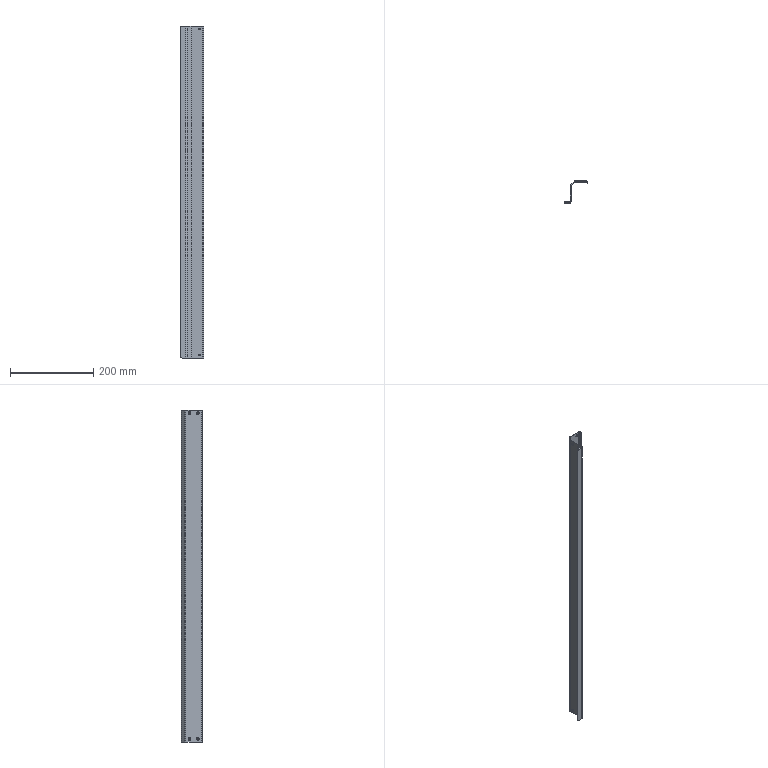Part | STEP file | In/out guide rail cover plate 1 | 1 solid | 36 faces | box 57 x 52 x 800 mm | volume 124915 mm3 | plane 14 | cone 12 | cylinder 10 | commonest cylinder face diameters 3 x4 6 x4 10 x2
STEP:
#1=CARTESIAN_POINT('',(258.,43.5,390.639));
#2=VERTEX_POINT('',#1);
#3=CARTESIAN_POINT('',(258.,43.5,394.361));
#4=VERTEX_POINT('',#3);
#5=CARTESIAN_POINT('',(258.,43.5,392.5));
#6=DIRECTION('',(0.,1.,0.));
#7=DIRECTION('',(0.,0.,1.));
#8=AXIS2_PLACEMENT_3D('',#5,#6,#7);
#9=CIRCLE('',#8,1.861);
#10=EDGE_CURVE('',#2,#4,#9,.T.);
#11=ORIENTED_EDGE('',*,*,#10,.F.);
#12=CARTESIAN_POINT('',(258.,45.,389.14));
#13=VERTEX_POINT('',#12);
#14=CARTESIAN_POINT('',(258.,45.,389.14));
#15=DIRECTION('',(0.,0.7073,-0.7069));
#16=VECTOR('',#15,1000.);
#17=LINE('',#14,#16);
#18=EDGE_CURVE('',#2,#13,#17,.T.);
#19=ORIENTED_EDGE('',*,*,#18,.T.);
#20=CARTESIAN_POINT('',(258.,45.,395.86));
#21=VERTEX_POINT('',#20);
#22=CARTESIAN_POINT('',(258.,45.,392.5));
#23=DIRECTION('',(0.,1.,0.));
#24=DIRECTION('',(0.,0.,1.));
#25=AXIS2_PLACEMENT_3D('',#22,#23,#24);
#26=CIRCLE('',#25,3.36);
#27=EDGE_CURVE('',#13,#21,#26,.T.);
#28=ORIENTED_EDGE('',*,*,#27,.T.);
#29=CARTESIAN_POINT('',(258.,45.,395.86));
#30=DIRECTION('',(0.,0.7073,0.7069));
#31=VECTOR('',#30,1000.);
#32=LINE('',#29,#31);
#33=EDGE_CURVE('',#4,#21,#32,.T.);
#34=ORIENTED_EDGE('',*,*,#33,.F.);
#35=EDGE_LOOP('',(#11,#19,#28,#34));
#36=FACE_OUTER_BOUND('',#35,.T.);
#37=CARTESIAN_POINT('',(258.,45.,392.5));
#38=DIRECTION('',(0.,1.,0.));
#39=DIRECTION('',(0.,0.,1.));
#40=AXIS2_PLACEMENT_3D('',#37,#38,#39);
#41=CONICAL_SURFACE('',#40,3.36,0.7851);
#42=ADVANCED_FACE('',(#36),#41,.F.);
#43=CARTESIAN_POINT('',(258.,43.5,-394.361));
#44=VERTEX_POINT('',#43);
#45=CARTESIAN_POINT('',(258.,43.5,-390.639));
#46=VERTEX_POINT('',#45);
#47=CARTESIAN_POINT('',(258.,43.5,-392.5));
#48=DIRECTION('',(0.,1.,0.));
#49=DIRECTION('',(0.,0.,1.));
#50=AXIS2_PLACEMENT_3D('',#47,#48,#49);
#51=CIRCLE('',#50,1.861);
#52=EDGE_CURVE('',#44,#46,#51,.T.);
#53=ORIENTED_EDGE('',*,*,#52,.F.);
#54=CARTESIAN_POINT('',(258.,45.,-395.86));
#55=VERTEX_POINT('',#54);
#56=CARTESIAN_POINT('',(258.,45.,-395.86));
#57=DIRECTION('',(0.,0.7073,-0.7069));
#58=VECTOR('',#57,1000.);
#59=LINE('',#56,#58);
#60=EDGE_CURVE('',#44,#55,#59,.T.);
#61=ORIENTED_EDGE('',*,*,#60,.T.);
#62=CARTESIAN_POINT('',(258.,45.,-389.14));
#63=VERTEX_POINT('',#62);
#64=CARTESIAN_POINT('',(258.,45.,-392.5));
#65=DIRECTION('',(0.,1.,0.));
#66=DIRECTION('',(0.,0.,1.));
#67=AXIS2_PLACEMENT_3D('',#64,#65,#66);
#68=CIRCLE('',#67,3.36);
#69=EDGE_CURVE('',#55,#63,#68,.T.);
#70=ORIENTED_EDGE('',*,*,#69,.T.);
#71=CARTESIAN_POINT('',(258.,45.,-389.14));
#72=DIRECTION('',(0.,0.7073,0.7069));
#73=VECTOR('',#72,1000.);
#74=LINE('',#71,#73);
#75=EDGE_CURVE('',#46,#63,#74,.T.);
#76=ORIENTED_EDGE('',*,*,#75,.F.);
#77=EDGE_LOOP('',(#53,#61,#70,#76));
#78=FACE_OUTER_BOUND('',#77,.T.);
#79=CARTESIAN_POINT('',(258.,45.,-392.5));
#80=DIRECTION('',(0.,1.,0.));
#81=DIRECTION('',(0.,0.,1.));
#82=AXIS2_PLACEMENT_3D('',#79,#80,#81);
#83=CONICAL_SURFACE('',#82,3.36,0.7851);
#84=ADVANCED_FACE('',(#78),#83,.F.);
#85=CARTESIAN_POINT('',(227.5,5.,390.639));
#86=VERTEX_POINT('',#85);
#87=CARTESIAN_POINT('',(227.5,5.,394.361));
#88=VERTEX_POINT('',#87);
#89=CARTESIAN_POINT('',(227.5,5.,392.5));
#90=DIRECTION('',(-1.,0.,0.));
#91=DIRECTION('',(0.,0.,1.));
#92=AXIS2_PLACEMENT_3D('',#89,#90,#91);
#93=CIRCLE('',#92,1.861);
#94=EDGE_CURVE('',#86,#88,#93,.T.);
#95=ORIENTED_EDGE('',*,*,#94,.F.);
#96=CARTESIAN_POINT('',(226.,5.,389.14));
#97=VERTEX_POINT('',#96);
#98=CARTESIAN_POINT('',(226.,5.,389.14));
#99=DIRECTION('',(-0.7073,0.,-0.7069));
#100=VECTOR('',#99,1000.);
#101=LINE('',#98,#100);
#102=EDGE_CURVE('',#86,#97,#101,.T.);
#103=ORIENTED_EDGE('',*,*,#102,.T.);
#104=CARTESIAN_POINT('',(226.,5.,395.86));
#105=VERTEX_POINT('',#104);
#106=CARTESIAN_POINT('',(226.,5.,392.5));
#107=DIRECTION('',(-1.,0.,0.));
#108=DIRECTION('',(0.,0.,1.));
#109=AXIS2_PLACEMENT_3D('',#106,#107,#108);
#110=CIRCLE('',#109,3.36);
#111=EDGE_CURVE('',#97,#105,#110,.T.);
#112=ORIENTED_EDGE('',*,*,#111,.T.);
#113=CARTESIAN_POINT('',(226.,5.,395.86));
#114=DIRECTION('',(-0.7073,0.,0.7069));
#115=VECTOR('',#114,1000.);
#116=LINE('',#113,#115);
#117=EDGE_CURVE('',#88,#105,#116,.T.);
#118=ORIENTED_EDGE('',*,*,#117,.F.);
#119=EDGE_LOOP('',(#95,#103,#112,#118));
#120=FACE_OUTER_BOUND('',#119,.T.);
#121=CARTESIAN_POINT('',(226.,5.,392.5));
#122=DIRECTION('',(-1.,0.,0.));
#123=DIRECTION('',(0.,0.,1.));
#124=AXIS2_PLACEMENT_3D('',#121,#122,#123);
#125=CONICAL_SURFACE('',#124,3.36,0.7851);
#126=ADVANCED_FACE('',(#120),#125,.F.);
#127=CARTESIAN_POINT('',(227.5,5.,-394.361));
#128=VERTEX_POINT('',#127);
#129=CARTESIAN_POINT('',(227.5,5.,-390.639));
#130=VERTEX_POINT('',#129);
#131=CARTESIAN_POINT('',(227.5,5.,-392.5));
#132=DIRECTION('',(-1.,0.,0.));
#133=DIRECTION('',(0.,0.,1.));
#134=AXIS2_PLACEMENT_3D('',#131,#132,#133);
#135=CIRCLE('',#134,1.861);
#136=EDGE_CURVE('',#128,#130,#135,.T.);
#137=ORIENTED_EDGE('',*,*,#136,.F.);
#138=CARTESIAN_POINT('',(226.,5.,-395.86));
#139=VERTEX_POINT('',#138);
#140=CARTESIAN_POINT('',(226.,5.,-395.86));
#141=DIRECTION('',(-0.7073,0.,-0.7069));
#142=VECTOR('',#141,1000.);
#143=LINE('',#140,#142);
#144=EDGE_CURVE('',#128,#139,#143,.T.);
#145=ORIENTED_EDGE('',*,*,#144,.T.);
#146=CARTESIAN_POINT('',(226.,5.,-389.14));
#147=VERTEX_POINT('',#146);
#148=CARTESIAN_POINT('',(226.,5.,-392.5));
#149=DIRECTION('',(-1.,0.,0.));
#150=DIRECTION('',(0.,0.,1.));
#151=AXIS2_PLACEMENT_3D('',#148,#149,#150);
#152=CIRCLE('',#151,3.36);
#153=EDGE_CURVE('',#139,#147,#152,.T.);
#154=ORIENTED_EDGE('',*,*,#153,.T.);
#155=CARTESIAN_POINT('',(226.,5.,-389.14));
#156=DIRECTION('',(-0.7073,0.,0.7069));
#157=VECTOR('',#156,1000.);
#158=LINE('',#155,#157);
#159=EDGE_CURVE('',#130,#147,#158,.T.);
#160=ORIENTED_EDGE('',*,*,#159,.F.);
#161=EDGE_LOOP('',(#137,#145,#154,#160));
#162=FACE_OUTER_BOUND('',#161,.T.);
#163=CARTESIAN_POINT('',(226.,5.,-392.5));
#164=DIRECTION('',(-1.,0.,0.));
#165=DIRECTION('',(0.,0.,1.));
#166=AXIS2_PLACEMENT_3D('',#163,#164,#165);
#167=CONICAL_SURFACE('',#166,3.36,0.7851);
#168=ADVANCED_FACE('',(#162),#167,.F.);
#169=CARTESIAN_POINT('',(227.5,25.,-394.361));
#170=VERTEX_POINT('',#169);
#171=CARTESIAN_POINT('',(227.5,25.,-390.639));
#172=VERTEX_POINT('',#171);
#173=CARTESIAN_POINT('',(227.5,25.,-392.5));
#174=DIRECTION('',(-1.,0.,0.));
#175=DIRECTION('',(0.,0.,1.));
#176=AXIS2_PLACEMENT_3D('',#173,#174,#175);
#177=CIRCLE('',#176,1.861);
#178=EDGE_CURVE('',#170,#172,#177,.T.);
#179=ORIENTED_EDGE('',*,*,#178,.F.);
#180=CARTESIAN_POINT('',(226.,25.,-395.86));
#181=VERTEX_POINT('',#180);
#182=CARTESIAN_POINT('',(226.,25.,-395.86));
#183=DIRECTION('',(-0.7073,0.,-0.7069));
#184=VECTOR('',#183,1000.);
#185=LINE('',#182,#184);
#186=EDGE_CURVE('',#170,#181,#185,.T.);
#187=ORIENTED_EDGE('',*,*,#186,.T.);
#188=CARTESIAN_POINT('',(226.,25.,-389.14));
#189=VERTEX_POINT('',#188);
#190=CARTESIAN_POINT('',(226.,25.,-392.5));
#191=DIRECTION('',(-1.,0.,0.));
#192=DIRECTION('',(0.,0.,1.));
#193=AXIS2_PLACEMENT_3D('',#190,#191,#192);
#194=CIRCLE('',#193,3.36);
#195=EDGE_CURVE('',#181,#189,#194,.T.);
#196=ORIENTED_EDGE('',*,*,#195,.T.);
#197=CARTESIAN_POINT('',(226.,25.,-389.14));
#198=DIRECTION('',(-0.7073,0.,0.7069));
#199=VECTOR('',#198,1000.);
#200=LINE('',#197,#199);
#201=EDGE_CURVE('',#172,#189,#200,.T.);
#202=ORIENTED_EDGE('',*,*,#201,.F.);
#203=EDGE_LOOP('',(#179,#187,#196,#202));
#204=FACE_OUTER_BOUND('',#203,.T.);
#205=CARTESIAN_POINT('',(226.,25.,-392.5));
#206=DIRECTION('',(-1.,0.,0.));
#207=DIRECTION('',(0.,0.,1.));
#208=AXIS2_PLACEMENT_3D('',#205,#206,#207);
#209=CONICAL_SURFACE('',#208,3.36,0.7851);
#210=ADVANCED_FACE('',(#204),#209,.F.);
#211=CARTESIAN_POINT('',(227.5,25.,390.639));
#212=VERTEX_POINT('',#211);
#213=CARTESIAN_POINT('',(227.5,25.,394.361));
#214=VERTEX_POINT('',#213);
#215=CARTESIAN_POINT('',(227.5,25.,392.5));
#216=DIRECTION('',(-1.,0.,0.));
#217=DIRECTION('',(0.,0.,1.));
#218=AXIS2_PLACEMENT_3D('',#215,#216,#217);
#219=CIRCLE('',#218,1.861);
#220=EDGE_CURVE('',#212,#214,#219,.T.);
#221=ORIENTED_EDGE('',*,*,#220,.F.);
#222=CARTESIAN_POINT('',(226.,25.,389.14));
#223=VERTEX_POINT('',#222);
#224=CARTESIAN_POINT('',(226.,25.,389.14));
#225=DIRECTION('',(-0.7073,0.,-0.7069));
#226=VECTOR('',#225,1000.);
#227=LINE('',#224,#226);
#228=EDGE_CURVE('',#212,#223,#227,.T.);
#229=ORIENTED_EDGE('',*,*,#228,.T.);
#230=CARTESIAN_POINT('',(226.,25.,395.86));
#231=VERTEX_POINT('',#230);
#232=CARTESIAN_POINT('',(226.,25.,392.5));
#233=DIRECTION('',(-1.,0.,0.));
#234=DIRECTION('',(0.,0.,1.));
#235=AXIS2_PLACEMENT_3D('',#232,#233,#234);
#236=CIRCLE('',#235,3.36);
#237=EDGE_CURVE('',#223,#231,#236,.T.);
#238=ORIENTED_EDGE('',*,*,#237,.T.);
#239=CARTESIAN_POINT('',(226.,25.,395.86));
#240=DIRECTION('',(-0.7073,0.,0.7069));
#241=VECTOR('',#240,1000.);
#242=LINE('',#239,#241);
#243=EDGE_CURVE('',#214,#231,#242,.T.);
#244=ORIENTED_EDGE('',*,*,#243,.F.);
#245=EDGE_LOOP('',(#221,#229,#238,#244));
#246=FACE_OUTER_BOUND('',#245,.T.);
#247=CARTESIAN_POINT('',(226.,25.,392.5));
#248=DIRECTION('',(-1.,0.,0.));
#249=DIRECTION('',(0.,0.,1.));
#250=AXIS2_PLACEMENT_3D('',#247,#248,#249);
#251=CONICAL_SURFACE('',#250,3.36,0.7851);
#252=ADVANCED_FACE('',(#246),#251,.F.);
#253=CARTESIAN_POINT('',(258.,43.5,392.5));
#254=DIRECTION('',(0.,1.,0.));
#255=DIRECTION('',(0.,0.,1.));
#256=AXIS2_PLACEMENT_3D('',#253,#254,#255);
#257=CIRCLE('',#256,1.861);
#258=EDGE_CURVE('',#4,#2,#257,.T.);
#259=ORIENTED_EDGE('',*,*,#258,.T.);
#260=ORIENTED_EDGE('',*,*,#10,.T.);
#261=EDGE_LOOP('',(#259,#260));
#262=FACE_BOUND('',#261,.T.);
#263=CARTESIAN_POINT('',(258.,43.5,-392.5));
#264=DIRECTION('',(0.,1.,0.));
#265=DIRECTION('',(0.,0.,1.));
#266=AXIS2_PLACEMENT_3D('',#263,#264,#265);
#267=CIRCLE('',#266,1.861);
#268=EDGE_CURVE('',#46,#44,#267,.T.);
#269=ORIENTED_EDGE('',*,*,#268,.T.);
#270=ORIENTED_EDGE('',*,*,#52,.T.);
#271=EDGE_LOOP('',(#269,#270));
#272=FACE_BOUND('',#271,.T.);
#273=CARTESIAN_POINT('',(265.,43.5,-400.));
#274=VERTEX_POINT('',#273);
#275=CARTESIAN_POINT('',(237.243,43.5,-400.));
#276=VERTEX_POINT('',#275);
#277=CARTESIAN_POINT('',(0.,43.5,-400.));
#278=DIRECTION('',(-1.,0.,0.));
#279=VECTOR('',#278,1000.);
#280=LINE('',#277,#279);
#281=EDGE_CURVE('',#274,#276,#280,.T.);
#282=ORIENTED_EDGE('',*,*,#281,.F.);
#283=CARTESIAN_POINT('',(265.,43.5,400.));
#284=VERTEX_POINT('',#283);
#285=CARTESIAN_POINT('',(265.,43.5,400.));
#286=DIRECTION('',(0.,0.,1.));
#287=VECTOR('',#286,1000.);
#288=LINE('',#285,#287);
#289=EDGE_CURVE('',#274,#284,#288,.T.);
#290=ORIENTED_EDGE('',*,*,#289,.T.);
#291=CARTESIAN_POINT('',(237.243,43.5,400.));
#292=VERTEX_POINT('',#291);
#293=CARTESIAN_POINT('',(268.,43.5,400.));
#294=DIRECTION('',(-1.,0.,0.));
#295=VECTOR('',#294,1000.);
#296=LINE('',#293,#295);
#297=EDGE_CURVE('',#284,#292,#296,.T.);
#298=ORIENTED_EDGE('',*,*,#297,.T.);
#299=CARTESIAN_POINT('',(237.243,43.5,-400.));
#300=DIRECTION('',(0.,0.,-1.));
#301=VECTOR('',#300,1000.);
#302=LINE('',#299,#301);
#303=EDGE_CURVE('',#292,#276,#302,.T.);
#304=ORIENTED_EDGE('',*,*,#303,.T.);
#305=EDGE_LOOP('',(#282,#290,#298,#304));
#306=FACE_OUTER_BOUND('',#305,.T.);
#307=CARTESIAN_POINT('',(268.,43.5,-400.));
#308=DIRECTION('',(0.,1.,0.));
#309=DIRECTION('',(0.,0.,1.));
#310=AXIS2_PLACEMENT_3D('',#307,#308,#309);
#311=PLANE('',#310);
#312=ADVANCED_FACE('',(#262,#272,#306),#311,.F.);
#313=CARTESIAN_POINT('',(235.121,44.121,-400.));
#314=VERTEX_POINT('',#313);
#315=CARTESIAN_POINT('',(226.879,35.879,-400.));
#316=VERTEX_POINT('',#315);
#317=CARTESIAN_POINT('',(236.,45.,-400.));
#318=DIRECTION('',(-0.7071,-0.7071,0.));
#319=VECTOR('',#318,1000.);
#320=LINE('',#317,#319);
#321=EDGE_CURVE('',#314,#316,#320,.T.);
#322=ORIENTED_EDGE('',*,*,#321,.T.);
#323=CARTESIAN_POINT('',(226.879,35.879,400.));
#324=VERTEX_POINT('',#323);
#325=CARTESIAN_POINT('',(226.879,35.879,-400.));
#326=DIRECTION('',(0.,0.,1.));
#327=VECTOR('',#326,1000.);
#328=LINE('',#325,#327);
#329=EDGE_CURVE('',#316,#324,#328,.T.);
#330=ORIENTED_EDGE('',*,*,#329,.T.);
#331=CARTESIAN_POINT('',(235.121,44.121,400.));
#332=VERTEX_POINT('',#331);
#333=CARTESIAN_POINT('',(236.,45.,400.));
#334=DIRECTION('',(-0.7071,-0.7071,0.));
#335=VECTOR('',#334,1000.);
#336=LINE('',#333,#335);
#337=EDGE_CURVE('',#332,#324,#336,.T.);
#338=ORIENTED_EDGE('',*,*,#337,.F.);
#339=CARTESIAN_POINT('',(235.121,44.121,-400.));
#340=DIRECTION('',(0.,0.,-1.));
#341=VECTOR('',#340,1000.);
#342=LINE('',#339,#341);
#343=EDGE_CURVE('',#332,#314,#342,.T.);
#344=ORIENTED_EDGE('',*,*,#343,.T.);
#345=EDGE_LOOP('',(#322,#330,#338,#344));
#346=FACE_OUTER_BOUND('',#345,.T.);
#347=CARTESIAN_POINT('',(236.,45.,-400.));
#348=DIRECTION('',(-0.7071,0.7071,0.));
#349=DIRECTION('',(-0.7071,-0.7071,0.));
#350=AXIS2_PLACEMENT_3D('',#347,#348,#349);
#351=PLANE('',#350);
#352=ADVANCED_FACE('',(#346),#351,.T.);
#353=CARTESIAN_POINT('',(258.,45.,392.5));
#354=DIRECTION('',(0.,1.,0.));
#355=DIRECTION('',(0.,0.,1.));
#356=AXIS2_PLACEMENT_3D('',#353,#354,#355);
#357=CIRCLE('',#356,3.36);
#358=EDGE_CURVE('',#21,#13,#357,.T.);
#359=ORIENTED_EDGE('',*,*,#358,.F.);
#360=ORIENTED_EDGE('',*,*,#27,.F.);
#361=EDGE_LOOP('',(#359,#360));
#362=FACE_BOUND('',#361,.T.);
#363=CARTESIAN_POINT('',(258.,45.,-392.5));
#364=DIRECTION('',(0.,1.,0.));
#365=DIRECTION('',(0.,0.,1.));
#366=AXIS2_PLACEMENT_3D('',#363,#364,#365);
#367=CIRCLE('',#366,3.36);
#368=EDGE_CURVE('',#63,#55,#367,.T.);
#369=ORIENTED_EDGE('',*,*,#368,.F.);
#370=ORIENTED_EDGE('',*,*,#69,.F.);
#371=EDGE_LOOP('',(#369,#370));
#372=FACE_BOUND('',#371,.T.);
#373=CARTESIAN_POINT('',(265.,45.,-400.));
#374=VERTEX_POINT('',#373);
#375=CARTESIAN_POINT('',(237.243,45.,-400.));
#376=VERTEX_POINT('',#375);
#377=CARTESIAN_POINT('',(268.,45.,-400.));
#378=DIRECTION('',(-1.,0.,0.));
#379=VECTOR('',#378,1000.);
#380=LINE('',#377,#379);
#381=EDGE_CURVE('',#374,#376,#380,.T.);
#382=ORIENTED_EDGE('',*,*,#381,.T.);
#383=CARTESIAN_POINT('',(237.243,45.,400.));
#384=VERTEX_POINT('',#383);
#385=CARTESIAN_POINT('',(237.243,45.,-400.));
#386=DIRECTION('',(0.,0.,1.));
#387=VECTOR('',#386,1000.);
#388=LINE('',#385,#387);
#389=EDGE_CURVE('',#376,#384,#388,.T.);
#390=ORIENTED_EDGE('',*,*,#389,.T.);
#391=CARTESIAN_POINT('',(265.,45.,400.));
#392=VERTEX_POINT('',#391);
#393=CARTESIAN_POINT('',(268.,45.,400.));
#394=DIRECTION('',(-1.,0.,0.));
#395=VECTOR('',#394,1000.);
#396=LINE('',#393,#395);
#397=EDGE_CURVE('',#392,#384,#396,.T.);
#398=ORIENTED_EDGE('',*,*,#397,.F.);
#399=CARTESIAN_POINT('',(265.,45.,-400.));
#400=DIRECTION('',(0.,0.,-1.));
#401=VECTOR('',#400,1000.);
#402=LINE('',#399,#401);
#403=EDGE_CURVE('',#392,#374,#402,.T.);
#404=ORIENTED_EDGE('',*,*,#403,.T.);
#405=EDGE_LOOP('',(#382,#390,#398,#404));
#406=FACE_OUTER_BOUND('',#405,.T.);
#407=CARTESIAN_POINT('',(268.,45.,-400.));
#408=DIRECTION('',(0.,1.,0.));
#409=DIRECTION('',(0.,0.,1.));
#410=AXIS2_PLACEMENT_3D('',#407,#408,#409);
#411=PLANE('',#410);
#412=ADVANCED_FACE('',(#362,#372,#406),#411,.T.);
#413=CARTESIAN_POINT('',(268.,39.,-400.));
#414=VERTEX_POINT('',#413);
#415=CARTESIAN_POINT('',(268.,42.,-400.));
#416=VERTEX_POINT('',#415);
#417=CARTESIAN_POINT('',(268.,-7.,-400.));
#418=DIRECTION('',(0.,1.,0.));
#419=VECTOR('',#418,1000.);
#420=LINE('',#417,#419);
#421=EDGE_CURVE('',#414,#416,#420,.T.);
#422=ORIENTED_EDGE('',*,*,#421,.T.);
#423=CARTESIAN_POINT('',(268.,42.,400.));
#424=VERTEX_POINT('',#423);
#425=CARTESIAN_POINT('',(268.,42.,-400.));
#426=DIRECTION('',(0.,0.,1.));
#427=VECTOR('',#426,1000.);
#428=LINE('',#425,#427);
#429=EDGE_CURVE('',#416,#424,#428,.T.);
#430=ORIENTED_EDGE('',*,*,#429,.T.);
#431=CARTESIAN_POINT('',(268.,39.,400.));
#432=VERTEX_POINT('',#431);
#433=CARTESIAN_POINT('',(268.,-7.,400.));
#434=DIRECTION('',(0.,1.,0.));
#435=VECTOR('',#434,1000.);
#436=LINE('',#433,#435);
#437=EDGE_CURVE('',#432,#424,#436,.T.);
#438=ORIENTED_EDGE('',*,*,#437,.F.);
#439=CARTESIAN_POINT('',(268.,39.,400.));
#440=DIRECTION('',(0.,0.,1.));
#441=VECTOR('',#440,1000.);
#442=LINE('',#439,#441);
#443=EDGE_CURVE('',#414,#432,#442,.T.);
#444=ORIENTED_EDGE('',*,*,#443,.F.);
#445=EDGE_LOOP('',(#422,#430,#438,#444));
#446=FACE_OUTER_BOUND('',#445,.T.);
#447=CARTESIAN_POINT('',(268.,-7.,-400.));
#448=DIRECTION('',(1.,0.,0.));
#449=DIRECTION('',(0.,0.,-1.));
#450=AXIS2_PLACEMENT_3D('',#447,#448,#449);
#451=PLANE('',#450);
#452=ADVANCED_FACE('',(#446),#451,.T.);
#453=CARTESIAN_POINT('',(216.,-7.,400.));
#454=VERTEX_POINT('',#453);
#455=CARTESIAN_POINT('',(224.5,-7.,400.));
#456=VERTEX_POINT('',#455);
#457=CARTESIAN_POINT('',(226.,-7.,400.));
#458=DIRECTION('',(1.,0.,0.));
#459=VECTOR('',#458,1000.);
#460=LINE('',#457,#459);
#461=EDGE_CURVE('',#454,#456,#460,.T.);
#462=ORIENTED_EDGE('',*,*,#461,.F.);
#463=CARTESIAN_POINT('',(211.,-7.,395.));
#464=VERTEX_POINT('',#463);
#465=CARTESIAN_POINT('',(216.,-7.,395.));
#466=DIRECTION('',(0.,-1.,0.));
#467=DIRECTION('',(1.,0.,0.));
#468=AXIS2_PLACEMENT_3D('',#465,#466,#467);
#469=CIRCLE('',#468,5.);
#470=EDGE_CURVE('',#454,#464,#469,.T.);
#471=ORIENTED_EDGE('',*,*,#470,.T.);
#472=CARTESIAN_POINT('',(211.,-7.,-395.));
#473=VERTEX_POINT('',#472);
#474=CARTESIAN_POINT('',(211.,-7.,400.));
#475=DIRECTION('',(0.,0.,1.));
#476=VECTOR('',#475,1000.);
#477=LINE('',#474,#476);
#478=EDGE_CURVE('',#473,#464,#477,.T.);
#479=ORIENTED_EDGE('',*,*,#478,.F.);
#480=CARTESIAN_POINT('',(216.,-7.,-400.));
#481=VERTEX_POINT('',#480);
#482=CARTESIAN_POINT('',(216.,-7.,-395.));
#483=DIRECTION('',(0.,-1.,0.));
#484=DIRECTION('',(1.,0.,0.));
#485=AXIS2_PLACEMENT_3D('',#482,#483,#484);
#486=CIRCLE('',#485,5.);
#487=EDGE_CURVE('',#473,#481,#486,.T.);
#488=ORIENTED_EDGE('',*,*,#487,.T.);
#489=CARTESIAN_POINT('',(224.5,-7.,-400.));
#490=VERTEX_POINT('',#489);
#491=CARTESIAN_POINT('',(226.,-7.,-400.));
#492=DIRECTION('',(1.,0.,0.));
#493=VECTOR('',#492,1000.);
#494=LINE('',#491,#493);
#495=EDGE_CURVE('',#481,#490,#494,.T.);
#496=ORIENTED_EDGE('',*,*,#495,.T.);
#497=CARTESIAN_POINT('',(224.5,-7.,400.));
#498=DIRECTION('',(0.,0.,1.));
#499=VECTOR('',#498,1000.);
#500=LINE('',#497,#499);
#501=EDGE_CURVE('',#490,#456,#500,.T.);
#502=ORIENTED_EDGE('',*,*,#501,.T.);
#503=EDGE_LOOP('',(#462,#471,#479,#488,#496,#502));
#504=FACE_OUTER_BOUND('',#503,.T.);
#505=CARTESIAN_POINT('',(226.,-7.,-400.));
#506=DIRECTION('',(0.,-1.,0.));
#507=DIRECTION('',(1.,0.,0.));
#508=AXIS2_PLACEMENT_3D('',#505,#506,#507);
#509=PLANE('',#508);
#510=ADVANCED_FACE('',(#504),#509,.T.);
#511=CARTESIAN_POINT('',(226.,5.,392.5));
#512=DIRECTION('',(-1.,0.,0.));
#513=DIRECTION('',(0.,0.,1.));
#514=AXIS2_PLACEMENT_3D('',#511,#512,#513);
#515=CIRCLE('',#514,3.36);
#516=EDGE_CURVE('',#105,#97,#515,.T.);
#517=ORIENTED_EDGE('',*,*,#516,.F.);
#518=ORIENTED_EDGE('',*,*,#111,.F.);
#519=EDGE_LOOP('',(#517,#518));
#520=FACE_BOUND('',#519,.T.);
#521=CARTESIAN_POINT('',(226.,5.,-392.5));
#522=DIRECTION('',(-1.,0.,0.));
#523=DIRECTION('',(0.,0.,1.));
#524=AXIS2_PLACEMENT_3D('',#521,#522,#523);
#525=CIRCLE('',#524,3.36);
#526=EDGE_CURVE('',#147,#139,#525,.T.);
#527=ORIENTED_EDGE('',*,*,#526,.F.);
#528=ORIENTED_EDGE('',*,*,#153,.F.);
#529=EDGE_LOOP('',(#527,#528));
#530=FACE_BOUND('',#529,.T.);
#531=CARTESIAN_POINT('',(226.,25.,-392.5));
#532=DIRECTION('',(-1.,0.,0.));
#533=DIRECTION('',(0.,0.,1.));
#534=AXIS2_PLACEMENT_3D('',#531,#532,#533);
#535=CIRCLE('',#534,3.36);
#536=EDGE_CURVE('',#189,#181,#535,.T.);
#537=ORIENTED_EDGE('',*,*,#536,.F.);
#538=ORIENTED_EDGE('',*,*,#195,.F.);
#539=EDGE_LOOP('',(#537,#538));
#540=FACE_BOUND('',#539,.T.);
#541=CARTESIAN_POINT('',(226.,25.,392.5));
#542=DIRECTION('',(-1.,0.,0.));
#543=DIRECTION('',(0.,0.,1.));
#544=AXIS2_PLACEMENT_3D('',#541,#542,#543);
#545=CIRCLE('',#544,3.36);
#546=EDGE_CURVE('',#231,#223,#545,.T.);
#547=ORIENTED_EDGE('',*,*,#546,.F.);
#548=ORIENTED_EDGE('',*,*,#237,.F.);
#549=EDGE_LOOP('',(#547,#548));
#550=FACE_BOUND('',#549,.T.);
#551=CARTESIAN_POINT('',(226.,33.757,400.));
#552=VERTEX_POINT('',#551);
#553=CARTESIAN_POINT('',(226.,-4.,400.));
#554=VERTEX_POINT('',#553);
#555=CARTESIAN_POINT('',(226.,35.,400.));
#556=DIRECTION('',(0.,-1.,0.));
#557=VECTOR('',#556,1000.);
#558=LINE('',#555,#557);
#559=EDGE_CURVE('',#552,#554,#558,.T.);
#560=ORIENTED_EDGE('',*,*,#559,.F.);
#561=CARTESIAN_POINT('',(226.,33.757,-400.));
#562=VERTEX_POINT('',#561);
#563=CARTESIAN_POINT('',(226.,33.757,-400.));
#564=DIRECTION('',(0.,0.,-1.));
#565=VECTOR('',#564,1000.);
#566=LINE('',#563,#565);
#567=EDGE_CURVE('',#552,#562,#566,.T.);
#568=ORIENTED_EDGE('',*,*,#567,.T.);
#569=CARTESIAN_POINT('',(226.,-4.,-400.));
#570=VERTEX_POINT('',#569);
#571=CARTESIAN_POINT('',(226.,35.,-400.));
#572=DIRECTION('',(0.,-1.,0.));
#573=VECTOR('',#572,1000.);
#574=LINE('',#571,#573);
#575=EDGE_CURVE('',#562,#570,#574,.T.);
#576=ORIENTED_EDGE('',*,*,#575,.T.);
#577=CARTESIAN_POINT('',(226.,-4.,-400.));
#578=DIRECTION('',(0.,0.,1.));
#579=VECTOR('',#578,1000.);
#580=LINE('',#577,#579);
#581=EDGE_CURVE('',#570,#554,#580,.T.);
#582=ORIENTED_EDGE('',*,*,#581,.T.);
#583=EDGE_LOOP('',(#560,#568,#576,#582));
#584=FACE_OUTER_BOUND('',#583,.T.);
#585=CARTESIAN_POINT('',(226.,35.,-400.));
#586=DIRECTION('',(-1.,0.,0.));
#587=DIRECTION('',(0.,0.,1.));
#588=AXIS2_PLACEMENT_3D('',#585,#586,#587);
#589=PLANE('',#588);
#590=ADVANCED_FACE('',(#520,#530,#540,#550,#584),#589,.T.);
#591=ORIENTED_EDGE('',*,*,#495,.F.);
#592=CARTESIAN_POINT('',(216.,-5.5,-400.));
#593=VERTEX_POINT('',#592);
#594=CARTESIAN_POINT('',(216.,0.,-400.));
#595=DIRECTION('',(0.,1.,0.));
#596=VECTOR('',#595,1000.);
#597=LINE('',#594,#596);
#598=EDGE_CURVE('',#481,#593,#597,.T.);
#599=ORIENTED_EDGE('',*,*,#598,.T.);
#600=CARTESIAN_POINT('',(224.5,-5.5,-400.));
#601=VERTEX_POINT('',#600);
#602=CARTESIAN_POINT('',(211.,-5.5,-400.));
#603=DIRECTION('',(1.,0.,0.));
#604=VECTOR('',#603,1000.);
#605=LINE('',#602,#604);
#606=EDGE_CURVE('',#593,#601,#605,.T.);
#607=ORIENTED_EDGE('',*,*,#606,.T.);
#608=CARTESIAN_POINT('',(224.5,-4.,-400.));
#609=DIRECTION('',(0.,0.,1.));
#610=DIRECTION('',(1.,0.,0.));
#611=AXIS2_PLACEMENT_3D('',#608,#609,#610);
#612=CIRCLE('',#611,1.5);
#613=EDGE_CURVE('',#601,#570,#612,.T.);
#614=ORIENTED_EDGE('',*,*,#613,.T.);
#615=ORIENTED_EDGE('',*,*,#575,.F.);
#616=CARTESIAN_POINT('',(229.,33.757,-400.));
#617=DIRECTION('',(0.,0.,-1.));
#618=DIRECTION('',(1.,0.,0.));
#619=AXIS2_PLACEMENT_3D('',#616,#617,#618);
#620=CIRCLE('',#619,3.);
#621=EDGE_CURVE('',#562,#316,#620,.T.);
#622=ORIENTED_EDGE('',*,*,#621,.T.);
#623=ORIENTED_EDGE('',*,*,#321,.F.);
#624=CARTESIAN_POINT('',(237.243,42.,-400.));
#625=DIRECTION('',(0.,0.,-1.));
#626=DIRECTION('',(1.,0.,0.));
#627=AXIS2_PLACEMENT_3D('',#624,#625,#626);
#628=CIRCLE('',#627,3.);
#629=EDGE_CURVE('',#314,#376,#628,.T.);
#630=ORIENTED_EDGE('',*,*,#629,.T.);
#631=ORIENTED_EDGE('',*,*,#381,.F.);
#632=CARTESIAN_POINT('',(265.,42.,-400.));
#633=DIRECTION('',(0.,0.,-1.));
#634=DIRECTION('',(1.,0.,0.));
#635=AXIS2_PLACEMENT_3D('',#632,#633,#634);
#636=CIRCLE('',#635,3.);
#637=EDGE_CURVE('',#374,#416,#636,.T.);
#638=ORIENTED_EDGE('',*,*,#637,.T.);
#639=ORIENTED_EDGE('',*,*,#421,.F.);
#640=CARTESIAN_POINT('',(266.5,39.,-400.));
#641=VERTEX_POINT('',#640);
#642=CARTESIAN_POINT('',(268.,39.,-400.));
#643=DIRECTION('',(1.,0.,0.));
#644=VECTOR('',#643,1000.);
#645=LINE('',#642,#644);
#646=EDGE_CURVE('',#641,#414,#645,.T.);
#647=ORIENTED_EDGE('',*,*,#646,.F.);
#648=CARTESIAN_POINT('',(266.5,42.,-400.));
#649=VERTEX_POINT('',#648);
#650=CARTESIAN_POINT('',(266.5,39.,-400.));
#651=DIRECTION('',(0.,1.,0.));
#652=VECTOR('',#651,1000.);
#653=LINE('',#650,#652);
#654=EDGE_CURVE('',#641,#649,#653,.T.);
#655=ORIENTED_EDGE('',*,*,#654,.T.);
#656=CARTESIAN_POINT('',(265.,42.,-400.));
#657=DIRECTION('',(0.,0.,1.));
#658=DIRECTION('',(1.,0.,0.));
#659=AXIS2_PLACEMENT_3D('',#656,#657,#658);
#660=CIRCLE('',#659,1.5);
#661=EDGE_CURVE('',#649,#274,#660,.T.);
#662=ORIENTED_EDGE('',*,*,#661,.T.);
#663=ORIENTED_EDGE('',*,*,#281,.T.);
#664=CARTESIAN_POINT('',(236.182,43.061,-400.));
#665=VERTEX_POINT('',#664);
#666=CARTESIAN_POINT('',(237.243,42.,-400.));
#667=DIRECTION('',(0.,0.,1.));
#668=DIRECTION('',(1.,0.,0.));
#669=AXIS2_PLACEMENT_3D('',#666,#667,#668);
#670=CIRCLE('',#669,1.5);
#671=EDGE_CURVE('',#276,#665,#670,.T.);
#672=ORIENTED_EDGE('',*,*,#671,.T.);
#673=CARTESIAN_POINT('',(227.939,34.818,-400.));
#674=VERTEX_POINT('',#673);
#675=CARTESIAN_POINT('',(96.561,-96.561,-400.));
#676=DIRECTION('',(-0.7071,-0.7071,0.));
#677=VECTOR('',#676,1000.);
#678=LINE('',#675,#677);
#679=EDGE_CURVE('',#665,#674,#678,.T.);
#680=ORIENTED_EDGE('',*,*,#679,.T.);
#681=CARTESIAN_POINT('',(227.5,33.757,-400.));
#682=VERTEX_POINT('',#681);
#683=CARTESIAN_POINT('',(229.,33.757,-400.));
#684=DIRECTION('',(0.,0.,1.));
#685=DIRECTION('',(1.,0.,0.));
#686=AXIS2_PLACEMENT_3D('',#683,#684,#685);
#687=CIRCLE('',#686,1.5);
#688=EDGE_CURVE('',#674,#682,#687,.T.);
#689=ORIENTED_EDGE('',*,*,#688,.T.);
#690=CARTESIAN_POINT('',(227.5,-4.,-400.));
#691=VERTEX_POINT('',#690);
#692=CARTESIAN_POINT('',(227.5,0.,-400.));
#693=DIRECTION('',(0.,-1.,0.));
#694=VECTOR('',#693,1000.);
#695=LINE('',#692,#694);
#696=EDGE_CURVE('',#682,#691,#695,.T.);
#697=ORIENTED_EDGE('',*,*,#696,.T.);
#698=CARTESIAN_POINT('',(224.5,-4.,-400.));
#699=DIRECTION('',(0.,0.,-1.));
#700=DIRECTION('',(1.,0.,0.));
#701=AXIS2_PLACEMENT_3D('',#698,#699,#700);
#702=CIRCLE('',#701,3.);
#703=EDGE_CURVE('',#691,#490,#702,.T.);
#704=ORIENTED_EDGE('',*,*,#703,.T.);
#705=EDGE_LOOP('',(#591,#599,#607,#614,#615,#622,#623,#630,#631,#638,#639,#647,#655,#662,#663,#672,#680,#689,#697,#704));
#706=FACE_OUTER_BOUND('',#705,.T.);
#707=CARTESIAN_POINT('',(0.,0.,-400.));
#708=DIRECTION('',(0.,0.,1.));
#709=DIRECTION('',(1.,0.,0.));
#710=AXIS2_PLACEMENT_3D('',#707,#708,#709);
#711=PLANE('',#710);
#712=ADVANCED_FACE('',(#706),#711,.F.);
#713=CARTESIAN_POINT('',(216.,-5.5,400.));
#714=VERTEX_POINT('',#713);
#715=CARTESIAN_POINT('',(224.5,-5.5,400.));
#716=VERTEX_POINT('',#715);
#717=CARTESIAN_POINT('',(211.,-5.5,400.));
#718=DIRECTION('',(1.,0.,0.));
#719=VECTOR('',#718,1000.);
#720=LINE('',#717,#719);
#721=EDGE_CURVE('',#714,#716,#720,.T.);
#722=ORIENTED_EDGE('',*,*,#721,.F.);
#723=CARTESIAN_POINT('',(216.,-7.,400.));
#724=DIRECTION('',(0.,-1.,0.));
#725=VECTOR('',#724,1000.);
#726=LINE('',#723,#725);
#727=EDGE_CURVE('',#714,#454,#726,.T.);
#728=ORIENTED_EDGE('',*,*,#727,.T.);
#729=ORIENTED_EDGE('',*,*,#461,.T.);
#730=CARTESIAN_POINT('',(227.5,-4.,400.));
#731=VERTEX_POINT('',#730);
#732=CARTESIAN_POINT('',(224.5,-4.,400.));
#733=DIRECTION('',(0.,0.,1.));
#734=DIRECTION('',(1.,0.,0.));
#735=AXIS2_PLACEMENT_3D('',#732,#733,#734);
#736=CIRCLE('',#735,3.);
#737=EDGE_CURVE('',#456,#731,#736,.T.);
#738=ORIENTED_EDGE('',*,*,#737,.T.);
#739=CARTESIAN_POINT('',(227.5,33.757,400.));
#740=VERTEX_POINT('',#739);
#741=CARTESIAN_POINT('',(227.5,34.379,400.));
#742=DIRECTION('',(0.,-1.,0.));
#743=VECTOR('',#742,1000.);
#744=LINE('',#741,#743);
#745=EDGE_CURVE('',#740,#731,#744,.T.);
#746=ORIENTED_EDGE('',*,*,#745,.F.);
#747=CARTESIAN_POINT('',(227.939,34.818,400.));
#748=VERTEX_POINT('',#747);
#749=CARTESIAN_POINT('',(229.,33.757,400.));
#750=DIRECTION('',(0.,0.,-1.));
#751=DIRECTION('',(1.,0.,0.));
#752=AXIS2_PLACEMENT_3D('',#749,#750,#751);
#753=CIRCLE('',#752,1.5);
#754=EDGE_CURVE('',#740,#748,#753,.T.);
#755=ORIENTED_EDGE('',*,*,#754,.T.);
#756=CARTESIAN_POINT('',(236.182,43.061,400.));
#757=VERTEX_POINT('',#756);
#758=CARTESIAN_POINT('',(236.621,43.5,400.));
#759=DIRECTION('',(-0.7071,-0.7071,0.));
#760=VECTOR('',#759,1000.);
#761=LINE('',#758,#760);
#762=EDGE_CURVE('',#757,#748,#761,.T.);
#763=ORIENTED_EDGE('',*,*,#762,.F.);
#764=CARTESIAN_POINT('',(237.243,42.,400.));
#765=DIRECTION('',(0.,0.,-1.));
#766=DIRECTION('',(1.,0.,0.));
#767=AXIS2_PLACEMENT_3D('',#764,#765,#766);
#768=CIRCLE('',#767,1.5);
#769=EDGE_CURVE('',#757,#292,#768,.T.);
#770=ORIENTED_EDGE('',*,*,#769,.T.);
#771=ORIENTED_EDGE('',*,*,#297,.F.);
#772=CARTESIAN_POINT('',(266.5,42.,400.));
#773=VERTEX_POINT('',#772);
#774=CARTESIAN_POINT('',(265.,42.,400.));
#775=DIRECTION('',(0.,0.,-1.));
#776=DIRECTION('',(1.,0.,0.));
#777=AXIS2_PLACEMENT_3D('',#774,#775,#776);
#778=CIRCLE('',#777,1.5);
#779=EDGE_CURVE('',#284,#773,#778,.T.);
#780=ORIENTED_EDGE('',*,*,#779,.T.);
#781=CARTESIAN_POINT('',(266.5,39.,400.));
#782=VERTEX_POINT('',#781);
#783=CARTESIAN_POINT('',(266.5,39.,400.));
#784=DIRECTION('',(0.,1.,0.));
#785=VECTOR('',#784,1000.);
#786=LINE('',#783,#785);
#787=EDGE_CURVE('',#782,#773,#786,.T.);
#788=ORIENTED_EDGE('',*,*,#787,.F.);
#789=CARTESIAN_POINT('',(266.5,39.,400.));
#790=DIRECTION('',(-1.,0.,0.));
#791=VECTOR('',#790,1000.);
#792=LINE('',#789,#791);
#793=EDGE_CURVE('',#432,#782,#792,.T.);
#794=ORIENTED_EDGE('',*,*,#793,.F.);
#795=ORIENTED_EDGE('',*,*,#437,.T.);
#796=CARTESIAN_POINT('',(265.,42.,400.));
#797=DIRECTION('',(0.,0.,1.));
#798=DIRECTION('',(1.,0.,0.));
#799=AXIS2_PLACEMENT_3D('',#796,#797,#798);
#800=CIRCLE('',#799,3.);
#801=EDGE_CURVE('',#424,#392,#800,.T.);
#802=ORIENTED_EDGE('',*,*,#801,.T.);
#803=ORIENTED_EDGE('',*,*,#397,.T.);
#804=CARTESIAN_POINT('',(237.243,42.,400.));
#805=DIRECTION('',(0.,0.,1.));
#806=DIRECTION('',(1.,0.,0.));
#807=AXIS2_PLACEMENT_3D('',#804,#805,#806);
#808=CIRCLE('',#807,3.);
#809=EDGE_CURVE('',#384,#332,#808,.T.);
#810=ORIENTED_EDGE('',*,*,#809,.T.);
#811=ORIENTED_EDGE('',*,*,#337,.T.);
#812=CARTESIAN_POINT('',(229.,33.757,400.));
#813=DIRECTION('',(0.,0.,1.));
#814=DIRECTION('',(1.,0.,0.));
#815=AXIS2_PLACEMENT_3D('',#812,#813,#814);
#816=CIRCLE('',#815,3.);
#817=EDGE_CURVE('',#324,#552,#816,.T.);
#818=ORIENTED_EDGE('',*,*,#817,.T.);
#819=ORIENTED_EDGE('',*,*,#559,.T.);
#820=CARTESIAN_POINT('',(224.5,-4.,400.));
#821=DIRECTION('',(0.,0.,-1.));
#822=DIRECTION('',(1.,0.,0.));
#823=AXIS2_PLACEMENT_3D('',#820,#821,#822);
#824=CIRCLE('',#823,1.5);
#825=EDGE_CURVE('',#554,#716,#824,.T.);
#826=ORIENTED_EDGE('',*,*,#825,.T.);
#827=EDGE_LOOP('',(#722,#728,#729,#738,#746,#755,#763,#770,#771,#780,#788,#794,#795,#802,#803,#810,#811,#818,#819,#826));
#828=FACE_OUTER_BOUND('',#827,.T.);
#829=CARTESIAN_POINT('',(0.,0.,400.));
#830=DIRECTION('',(0.,0.,1.));
#831=DIRECTION('',(1.,0.,0.));
#832=AXIS2_PLACEMENT_3D('',#829,#830,#831);
#833=PLANE('',#832);
#834=ADVANCED_FACE('',(#828),#833,.T.);
#835=CARTESIAN_POINT('',(211.,-5.5,395.));
#836=VERTEX_POINT('',#835);
#837=CARTESIAN_POINT('',(211.,-5.5,-395.));
#838=VERTEX_POINT('',#837);
#839=CARTESIAN_POINT('',(211.,-5.5,-400.));
#840=DIRECTION('',(0.,0.,-1.));
#841=VECTOR('',#840,1000.);
#842=LINE('',#839,#841);
#843=EDGE_CURVE('',#836,#838,#842,.T.);
#844=ORIENTED_EDGE('',*,*,#843,.F.);
#845=CARTESIAN_POINT('',(216.,-5.5,395.));
#846=DIRECTION('',(0.,1.,0.));
#847=DIRECTION('',(0.,0.,-1.));
#848=AXIS2_PLACEMENT_3D('',#845,#846,#847);
#849=CIRCLE('',#848,5.);
#850=EDGE_CURVE('',#836,#714,#849,.T.);
#851=ORIENTED_EDGE('',*,*,#850,.T.);
#852=ORIENTED_EDGE('',*,*,#721,.T.);
#853=CARTESIAN_POINT('',(224.5,-5.5,-400.));
#854=DIRECTION('',(0.,0.,-1.));
#855=VECTOR('',#854,1000.);
#856=LINE('',#853,#855);
#857=EDGE_CURVE('',#716,#601,#856,.T.);
#858=ORIENTED_EDGE('',*,*,#857,.T.);
#859=ORIENTED_EDGE('',*,*,#606,.F.);
#860=CARTESIAN_POINT('',(216.,-5.5,-395.));
#861=DIRECTION('',(0.,1.,0.));
#862=DIRECTION('',(0.,0.,-1.));
#863=AXIS2_PLACEMENT_3D('',#860,#861,#862);
#864=CIRCLE('',#863,5.);
#865=EDGE_CURVE('',#593,#838,#864,.T.);
#866=ORIENTED_EDGE('',*,*,#865,.T.);
#867=EDGE_LOOP('',(#844,#851,#852,#858,#859,#866));
#868=FACE_OUTER_BOUND('',#867,.T.);
#869=CARTESIAN_POINT('',(211.,-5.5,-400.));
#870=DIRECTION('',(0.,-1.,0.));
#871=DIRECTION('',(0.,0.,-1.));
#872=AXIS2_PLACEMENT_3D('',#869,#870,#871);
#873=PLANE('',#872);
#874=ADVANCED_FACE('',(#868),#873,.F.);
#875=ORIENTED_EDGE('',*,*,#478,.T.);
#876=CARTESIAN_POINT('',(211.,-5.5,395.));
#877=DIRECTION('',(0.,1.,0.));
#878=VECTOR('',#877,1000.);
#879=LINE('',#876,#878);
#880=EDGE_CURVE('',#464,#836,#879,.T.);
#881=ORIENTED_EDGE('',*,*,#880,.T.);
#882=ORIENTED_EDGE('',*,*,#843,.T.);
#883=CARTESIAN_POINT('',(211.,0.,-395.));
#884=DIRECTION('',(0.,-1.,0.));
#885=VECTOR('',#884,1000.);
#886=LINE('',#883,#885);
#887=EDGE_CURVE('',#838,#473,#886,.T.);
#888=ORIENTED_EDGE('',*,*,#887,.T.);
#889=EDGE_LOOP('',(#875,#881,#882,#888));
#890=FACE_OUTER_BOUND('',#889,.T.);
#891=CARTESIAN_POINT('',(211.,0.,0.));
#892=DIRECTION('',(1.,0.,0.));
#893=DIRECTION('',(0.,0.,-1.));
#894=AXIS2_PLACEMENT_3D('',#891,#892,#893);
#895=PLANE('',#894);
#896=ADVANCED_FACE('',(#890),#895,.F.);
#897=CARTESIAN_POINT('',(227.5,5.,392.5));
#898=DIRECTION('',(-1.,0.,0.));
#899=DIRECTION('',(0.,0.,1.));
#900=AXIS2_PLACEMENT_3D('',#897,#898,#899);
#901=CIRCLE('',#900,1.861);
#902=EDGE_CURVE('',#88,#86,#901,.T.);
#903=ORIENTED_EDGE('',*,*,#902,.T.);
#904=ORIENTED_EDGE('',*,*,#94,.T.);
#905=EDGE_LOOP('',(#903,#904));
#906=FACE_BOUND('',#905,.T.);
#907=CARTESIAN_POINT('',(227.5,5.,-392.5));
#908=DIRECTION('',(-1.,0.,0.));
#909=DIRECTION('',(0.,0.,1.));
#910=AXIS2_PLACEMENT_3D('',#907,#908,#909);
#911=CIRCLE('',#910,1.861);
#912=EDGE_CURVE('',#130,#128,#911,.T.);
#913=ORIENTED_EDGE('',*,*,#912,.T.);
#914=ORIENTED_EDGE('',*,*,#136,.T.);
#915=EDGE_LOOP('',(#913,#914));
#916=FACE_BOUND('',#915,.T.);
#917=CARTESIAN_POINT('',(227.5,25.,-392.5));
#918=DIRECTION('',(-1.,0.,0.));
#919=DIRECTION('',(0.,0.,1.));
#920=AXIS2_PLACEMENT_3D('',#917,#918,#919);
#921=CIRCLE('',#920,1.861);
#922=EDGE_CURVE('',#172,#170,#921,.T.);
#923=ORIENTED_EDGE('',*,*,#922,.T.);
#924=ORIENTED_EDGE('',*,*,#178,.T.);
#925=EDGE_LOOP('',(#923,#924));
#926=FACE_BOUND('',#925,.T.);
#927=CARTESIAN_POINT('',(227.5,25.,392.5));
#928=DIRECTION('',(-1.,0.,0.));
#929=DIRECTION('',(0.,0.,1.));
#930=AXIS2_PLACEMENT_3D('',#927,#928,#929);
#931=CIRCLE('',#930,1.861);
#932=EDGE_CURVE('',#214,#212,#931,.T.);
#933=ORIENTED_EDGE('',*,*,#932,.T.);
#934=ORIENTED_EDGE('',*,*,#220,.T.);
#935=EDGE_LOOP('',(#933,#934));
#936=FACE_BOUND('',#935,.T.);
#937=ORIENTED_EDGE('',*,*,#745,.T.);
#938=CARTESIAN_POINT('',(227.5,-4.,-400.));
#939=DIRECTION('',(0.,0.,-1.));
#940=VECTOR('',#939,1000.);
#941=LINE('',#938,#940);
#942=EDGE_CURVE('',#731,#691,#941,.T.);
#943=ORIENTED_EDGE('',*,*,#942,.T.);
#944=ORIENTED_EDGE('',*,*,#696,.F.);
#945=CARTESIAN_POINT('',(227.5,33.757,400.));
#946=DIRECTION('',(0.,0.,1.));
#947=VECTOR('',#946,1000.);
#948=LINE('',#945,#947);
#949=EDGE_CURVE('',#682,#740,#948,.T.);
#950=ORIENTED_EDGE('',*,*,#949,.T.);
#951=EDGE_LOOP('',(#937,#943,#944,#950));
#952=FACE_OUTER_BOUND('',#951,.T.);
#953=CARTESIAN_POINT('',(227.5,34.379,-400.));
#954=DIRECTION('',(-1.,0.,0.));
#955=DIRECTION('',(0.,0.,1.));
#956=AXIS2_PLACEMENT_3D('',#953,#954,#955);
#957=PLANE('',#956);
#958=ADVANCED_FACE('',(#906,#916,#926,#936,#952),#957,.F.);
#959=ORIENTED_EDGE('',*,*,#679,.F.);
#960=CARTESIAN_POINT('',(236.182,43.061,400.));
#961=DIRECTION('',(0.,0.,1.));
#962=VECTOR('',#961,1000.);
#963=LINE('',#960,#962);
#964=EDGE_CURVE('',#665,#757,#963,.T.);
#965=ORIENTED_EDGE('',*,*,#964,.T.);
#966=ORIENTED_EDGE('',*,*,#762,.T.);
#967=CARTESIAN_POINT('',(227.939,34.818,-400.));
#968=DIRECTION('',(0.,0.,-1.));
#969=VECTOR('',#968,1000.);
#970=LINE('',#967,#969);
#971=EDGE_CURVE('',#748,#674,#970,.T.);
#972=ORIENTED_EDGE('',*,*,#971,.T.);
#973=EDGE_LOOP('',(#959,#965,#966,#972));
#974=FACE_OUTER_BOUND('',#973,.T.);
#975=CARTESIAN_POINT('',(236.621,43.5,-400.));
#976=DIRECTION('',(-0.7071,0.7071,0.));
#977=DIRECTION('',(-0.7071,-0.7071,0.));
#978=AXIS2_PLACEMENT_3D('',#975,#976,#977);
#979=PLANE('',#978);
#980=ADVANCED_FACE('',(#974),#979,.F.);
#981=ORIENTED_EDGE('',*,*,#787,.T.);
#982=CARTESIAN_POINT('',(266.5,42.,-400.));
#983=DIRECTION('',(0.,0.,-1.));
#984=VECTOR('',#983,1000.);
#985=LINE('',#982,#984);
#986=EDGE_CURVE('',#773,#649,#985,.T.);
#987=ORIENTED_EDGE('',*,*,#986,.T.);
#988=ORIENTED_EDGE('',*,*,#654,.F.);
#989=CARTESIAN_POINT('',(266.5,39.,-400.));
#990=DIRECTION('',(0.,0.,-1.));
#991=VECTOR('',#990,1000.);
#992=LINE('',#989,#991);
#993=EDGE_CURVE('',#782,#641,#992,.T.);
#994=ORIENTED_EDGE('',*,*,#993,.F.);
#995=EDGE_LOOP('',(#981,#987,#988,#994));
#996=FACE_OUTER_BOUND('',#995,.T.);
#997=CARTESIAN_POINT('',(266.5,39.,-400.));
#998=DIRECTION('',(1.,0.,0.));
#999=DIRECTION('',(0.,0.,-1.));
#1000=AXIS2_PLACEMENT_3D('',#997,#998,#999);
#1001=PLANE('',#1000);
#1002=ADVANCED_FACE('',(#996),#1001,.F.);
#1003=ORIENTED_EDGE('',*,*,#793,.T.);
#1004=ORIENTED_EDGE('',*,*,#993,.T.);
#1005=ORIENTED_EDGE('',*,*,#646,.T.);
#1006=ORIENTED_EDGE('',*,*,#443,.T.);
#1007=EDGE_LOOP('',(#1003,#1004,#1005,#1006));
#1008=FACE_OUTER_BOUND('',#1007,.T.);
#1009=CARTESIAN_POINT('',(0.,39.,0.));
#1010=DIRECTION('',(0.,1.,0.));
#1011=DIRECTION('',(0.,0.,1.));
#1012=AXIS2_PLACEMENT_3D('',#1009,#1010,#1011);
#1013=PLANE('',#1012);
#1014=ADVANCED_FACE('',(#1008),#1013,.F.);
#1015=ORIENTED_EDGE('',*,*,#228,.F.);
#1016=ORIENTED_EDGE('',*,*,#932,.F.);
#1017=ORIENTED_EDGE('',*,*,#243,.T.);
#1018=ORIENTED_EDGE('',*,*,#546,.T.);
#1019=EDGE_LOOP('',(#1015,#1016,#1017,#1018));
#1020=FACE_OUTER_BOUND('',#1019,.T.);
#1021=CARTESIAN_POINT('',(226.,25.,392.5));
#1022=DIRECTION('',(-1.,0.,0.));
#1023=DIRECTION('',(0.,0.,1.));
#1024=AXIS2_PLACEMENT_3D('',#1021,#1022,#1023);
#1025=CONICAL_SURFACE('',#1024,3.36,0.7851);
#1026=ADVANCED_FACE('',(#1020),#1025,.F.);
#1027=ORIENTED_EDGE('',*,*,#186,.F.);
#1028=ORIENTED_EDGE('',*,*,#922,.F.);
#1029=ORIENTED_EDGE('',*,*,#201,.T.);
#1030=ORIENTED_EDGE('',*,*,#536,.T.);
#1031=EDGE_LOOP('',(#1027,#1028,#1029,#1030));
#1032=FACE_OUTER_BOUND('',#1031,.T.);
#1033=CARTESIAN_POINT('',(226.,25.,-392.5));
#1034=DIRECTION('',(-1.,0.,0.));
#1035=DIRECTION('',(0.,0.,1.));
#1036=AXIS2_PLACEMENT_3D('',#1033,#1034,#1035);
#1037=CONICAL_SURFACE('',#1036,3.36,0.7851);
#1038=ADVANCED_FACE('',(#1032),#1037,.F.);
#1039=ORIENTED_EDGE('',*,*,#144,.F.);
#1040=ORIENTED_EDGE('',*,*,#912,.F.);
#1041=ORIENTED_EDGE('',*,*,#159,.T.);
#1042=ORIENTED_EDGE('',*,*,#526,.T.);
#1043=EDGE_LOOP('',(#1039,#1040,#1041,#1042));
#1044=FACE_OUTER_BOUND('',#1043,.T.);
#1045=CARTESIAN_POINT('',(226.,5.,-392.5));
#1046=DIRECTION('',(-1.,0.,0.));
#1047=DIRECTION('',(0.,0.,1.));
#1048=AXIS2_PLACEMENT_3D('',#1045,#1046,#1047);
#1049=CONICAL_SURFACE('',#1048,3.36,0.7851);
#1050=ADVANCED_FACE('',(#1044),#1049,.F.);
#1051=ORIENTED_EDGE('',*,*,#102,.F.);
#1052=ORIENTED_EDGE('',*,*,#902,.F.);
#1053=ORIENTED_EDGE('',*,*,#117,.T.);
#1054=ORIENTED_EDGE('',*,*,#516,.T.);
#1055=EDGE_LOOP('',(#1051,#1052,#1053,#1054));
#1056=FACE_OUTER_BOUND('',#1055,.T.);
#1057=CARTESIAN_POINT('',(226.,5.,392.5));
#1058=DIRECTION('',(-1.,0.,0.));
#1059=DIRECTION('',(0.,0.,1.));
#1060=AXIS2_PLACEMENT_3D('',#1057,#1058,#1059);
#1061=CONICAL_SURFACE('',#1060,3.36,0.7851);
#1062=ADVANCED_FACE('',(#1056),#1061,.F.);
#1063=ORIENTED_EDGE('',*,*,#60,.F.);
#1064=ORIENTED_EDGE('',*,*,#268,.F.);
#1065=ORIENTED_EDGE('',*,*,#75,.T.);
#1066=ORIENTED_EDGE('',*,*,#368,.T.);
#1067=EDGE_LOOP('',(#1063,#1064,#1065,#1066));
#1068=FACE_OUTER_BOUND('',#1067,.T.);
#1069=CARTESIAN_POINT('',(258.,45.,-392.5));
#1070=DIRECTION('',(0.,1.,0.));
#1071=DIRECTION('',(0.,0.,1.));
#1072=AXIS2_PLACEMENT_3D('',#1069,#1070,#1071);
#1073=CONICAL_SURFACE('',#1072,3.36,0.7851);
#1074=ADVANCED_FACE('',(#1068),#1073,.F.);
#1075=ORIENTED_EDGE('',*,*,#18,.F.);
#1076=ORIENTED_EDGE('',*,*,#258,.F.);
#1077=ORIENTED_EDGE('',*,*,#33,.T.);
#1078=ORIENTED_EDGE('',*,*,#358,.T.);
#1079=EDGE_LOOP('',(#1075,#1076,#1077,#1078));
#1080=FACE_OUTER_BOUND('',#1079,.T.);
#1081=CARTESIAN_POINT('',(258.,45.,392.5));
#1082=DIRECTION('',(0.,1.,0.));
#1083=DIRECTION('',(0.,0.,1.));
#1084=AXIS2_PLACEMENT_3D('',#1081,#1082,#1083);
#1085=CONICAL_SURFACE('',#1084,3.36,0.7851);
#1086=ADVANCED_FACE('',(#1080),#1085,.F.);
#1087=ORIENTED_EDGE('',*,*,#779,.F.);
#1088=ORIENTED_EDGE('',*,*,#289,.F.);
#1089=ORIENTED_EDGE('',*,*,#661,.F.);
#1090=ORIENTED_EDGE('',*,*,#986,.F.);
#1091=EDGE_LOOP('',(#1087,#1088,#1089,#1090));
#1092=FACE_OUTER_BOUND('',#1091,.T.);
#1093=CARTESIAN_POINT('',(265.,42.,-400.));
#1094=DIRECTION('',(0.,0.,1.));
#1095=DIRECTION('',(1.,0.,0.));
#1096=AXIS2_PLACEMENT_3D('',#1093,#1094,#1095);
#1097=CYLINDRICAL_SURFACE('',#1096,1.5);
#1098=ADVANCED_FACE('',(#1092),#1097,.F.);
#1099=ORIENTED_EDGE('',*,*,#825,.F.);
#1100=ORIENTED_EDGE('',*,*,#581,.F.);
#1101=ORIENTED_EDGE('',*,*,#613,.F.);
#1102=ORIENTED_EDGE('',*,*,#857,.F.);
#1103=EDGE_LOOP('',(#1099,#1100,#1101,#1102));
#1104=FACE_OUTER_BOUND('',#1103,.T.);
#1105=CARTESIAN_POINT('',(224.5,-4.,-400.));
#1106=DIRECTION('',(0.,0.,-1.));
#1107=DIRECTION('',(-1.,0.,0.));
#1108=AXIS2_PLACEMENT_3D('',#1105,#1106,#1107);
#1109=CYLINDRICAL_SURFACE('',#1108,1.5);
#1110=ADVANCED_FACE('',(#1104),#1109,.F.);
#1111=ORIENTED_EDGE('',*,*,#671,.F.);
#1112=ORIENTED_EDGE('',*,*,#303,.F.);
#1113=ORIENTED_EDGE('',*,*,#769,.F.);
#1114=ORIENTED_EDGE('',*,*,#964,.F.);
#1115=EDGE_LOOP('',(#1111,#1112,#1113,#1114));
#1116=FACE_OUTER_BOUND('',#1115,.T.);
#1117=CARTESIAN_POINT('',(237.243,42.,-400.));
#1118=DIRECTION('',(0.,0.,-1.));
#1119=DIRECTION('',(-1.,0.,0.));
#1120=AXIS2_PLACEMENT_3D('',#1117,#1118,#1119);
#1121=CYLINDRICAL_SURFACE('',#1120,1.5);
#1122=ADVANCED_FACE('',(#1116),#1121,.F.);
#1123=ORIENTED_EDGE('',*,*,#688,.F.);
#1124=ORIENTED_EDGE('',*,*,#971,.F.);
#1125=ORIENTED_EDGE('',*,*,#754,.F.);
#1126=ORIENTED_EDGE('',*,*,#949,.F.);
#1127=EDGE_LOOP('',(#1123,#1124,#1125,#1126));
#1128=FACE_OUTER_BOUND('',#1127,.T.);
#1129=CARTESIAN_POINT('',(229.,33.757,-400.));
#1130=DIRECTION('',(0.,0.,-1.));
#1131=DIRECTION('',(-1.,0.,0.));
#1132=AXIS2_PLACEMENT_3D('',#1129,#1130,#1131);
#1133=CYLINDRICAL_SURFACE('',#1132,1.5);
#1134=ADVANCED_FACE('',(#1128),#1133,.F.);
#1135=ORIENTED_EDGE('',*,*,#621,.F.);
#1136=ORIENTED_EDGE('',*,*,#567,.F.);
#1137=ORIENTED_EDGE('',*,*,#817,.F.);
#1138=ORIENTED_EDGE('',*,*,#329,.F.);
#1139=EDGE_LOOP('',(#1135,#1136,#1137,#1138));
#1140=FACE_OUTER_BOUND('',#1139,.T.);
#1141=CARTESIAN_POINT('',(229.,33.757,-400.));
#1142=DIRECTION('',(0.,0.,1.));
#1143=DIRECTION('',(1.,0.,0.));
#1144=AXIS2_PLACEMENT_3D('',#1141,#1142,#1143);
#1145=CYLINDRICAL_SURFACE('',#1144,3.);
#1146=ADVANCED_FACE('',(#1140),#1145,.T.);
#1147=ORIENTED_EDGE('',*,*,#703,.F.);
#1148=ORIENTED_EDGE('',*,*,#942,.F.);
#1149=ORIENTED_EDGE('',*,*,#737,.F.);
#1150=ORIENTED_EDGE('',*,*,#501,.F.);
#1151=EDGE_LOOP('',(#1147,#1148,#1149,#1150));
#1152=FACE_OUTER_BOUND('',#1151,.T.);
#1153=CARTESIAN_POINT('',(224.5,-4.,-400.));
#1154=DIRECTION('',(0.,0.,-1.));
#1155=DIRECTION('',(-1.,0.,0.));
#1156=AXIS2_PLACEMENT_3D('',#1153,#1154,#1155);
#1157=CYLINDRICAL_SURFACE('',#1156,3.);
#1158=ADVANCED_FACE('',(#1152),#1157,.T.);
#1159=ORIENTED_EDGE('',*,*,#629,.F.);
#1160=ORIENTED_EDGE('',*,*,#343,.F.);
#1161=ORIENTED_EDGE('',*,*,#809,.F.);
#1162=ORIENTED_EDGE('',*,*,#389,.F.);
#1163=EDGE_LOOP('',(#1159,#1160,#1161,#1162));
#1164=FACE_OUTER_BOUND('',#1163,.T.);
#1165=CARTESIAN_POINT('',(237.243,42.,-400.));
#1166=DIRECTION('',(0.,0.,1.));
#1167=DIRECTION('',(1.,0.,0.));
#1168=AXIS2_PLACEMENT_3D('',#1165,#1166,#1167);
#1169=CYLINDRICAL_SURFACE('',#1168,3.);
#1170=ADVANCED_FACE('',(#1164),#1169,.T.);
#1171=ORIENTED_EDGE('',*,*,#637,.F.);
#1172=ORIENTED_EDGE('',*,*,#403,.F.);
#1173=ORIENTED_EDGE('',*,*,#801,.F.);
#1174=ORIENTED_EDGE('',*,*,#429,.F.);
#1175=EDGE_LOOP('',(#1171,#1172,#1173,#1174));
#1176=FACE_OUTER_BOUND('',#1175,.T.);
#1177=CARTESIAN_POINT('',(265.,42.,-400.));
#1178=DIRECTION('',(0.,0.,1.));
#1179=DIRECTION('',(1.,0.,0.));
#1180=AXIS2_PLACEMENT_3D('',#1177,#1178,#1179);
#1181=CYLINDRICAL_SURFACE('',#1180,3.);
#1182=ADVANCED_FACE('',(#1176),#1181,.T.);
#1183=ORIENTED_EDGE('',*,*,#470,.F.);
#1184=ORIENTED_EDGE('',*,*,#727,.F.);
#1185=ORIENTED_EDGE('',*,*,#850,.F.);
#1186=ORIENTED_EDGE('',*,*,#880,.F.);
#1187=EDGE_LOOP('',(#1183,#1184,#1185,#1186));
#1188=FACE_OUTER_BOUND('',#1187,.T.);
#1189=CARTESIAN_POINT('',(216.,0.,395.));
#1190=DIRECTION('',(0.,-1.,0.));
#1191=DIRECTION('',(0.,0.,-1.));
#1192=AXIS2_PLACEMENT_3D('',#1189,#1190,#1191);
#1193=CYLINDRICAL_SURFACE('',#1192,5.);
#1194=ADVANCED_FACE('',(#1188),#1193,.T.);
#1195=ORIENTED_EDGE('',*,*,#865,.F.);
#1196=ORIENTED_EDGE('',*,*,#598,.F.);
#1197=ORIENTED_EDGE('',*,*,#487,.F.);
#1198=ORIENTED_EDGE('',*,*,#887,.F.);
#1199=EDGE_LOOP('',(#1195,#1196,#1197,#1198));
#1200=FACE_OUTER_BOUND('',#1199,.T.);
#1201=CARTESIAN_POINT('',(216.,0.,-395.));
#1202=DIRECTION('',(0.,-1.,0.));
#1203=DIRECTION('',(0.,0.,-1.));
#1204=AXIS2_PLACEMENT_3D('',#1201,#1202,#1203);
#1205=CYLINDRICAL_SURFACE('',#1204,5.);
#1206=ADVANCED_FACE('',(#1200),#1205,.T.);
#1207=CLOSED_SHELL('',(#42,#84,#126,#168,#210,#252,#312,#352,#412,#452,#510,#590,#712,#834,#874,#896,#958,#980,#1002,#1014,#1026,#1038,#1050,#1062,#1074,#1086,#1098,#1110,#1122,#1134,#1146,#1158,#1170,#1182,#1194,#1206));
#1208=MANIFOLD_SOLID_BREP('',#1207);
#1209=CARTESIAN_POINT('',(0.,0.,0.));
#1210=DIRECTION('',(0.,0.,1.));
#1211=DIRECTION('',(1.,0.,0.));
#1212=AXIS2_PLACEMENT_3D('',#1209,#1210,#1211);
#1213=(LENGTH_UNIT()NAMED_UNIT(*)SI_UNIT(.MILLI.,.METRE.));
#1214=UNCERTAINTY_MEASURE_WITH_UNIT(LENGTH_MEASURE(0.00001),#1213,'','');
#1215=(NAMED_UNIT(*)PLANE_ANGLE_UNIT()SI_UNIT($,.RADIAN.));
#1216=(NAMED_UNIT(*)SI_UNIT($,.STERADIAN.)SOLID_ANGLE_UNIT());
#1217=(GEOMETRIC_REPRESENTATION_CONTEXT(3)GLOBAL_UNCERTAINTY_ASSIGNED_CONTEXT((#1214))GLOBAL_UNIT_ASSIGNED_CONTEXT((#1213,#1215,#1216))REPRESENTATION_CONTEXT('',''));
#1218=ADVANCED_BREP_SHAPE_REPRESENTATION('',(#1208,#1212),#1217);